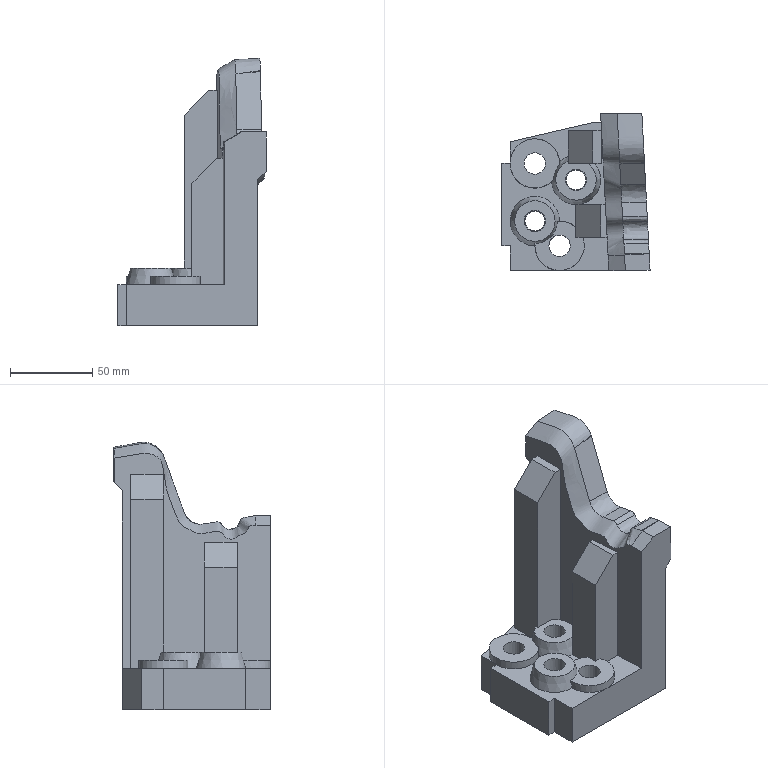Part | NX | features solid 2 | 1 solid | 65 faces | box 89.986 x 95.135 x 162.386 mm | volume 449307 mm3 | plane 34 | spline 17 | cylinder 10 | cone 4 | commonest cylinder face diameters 13 x4 30 x4 12 x2